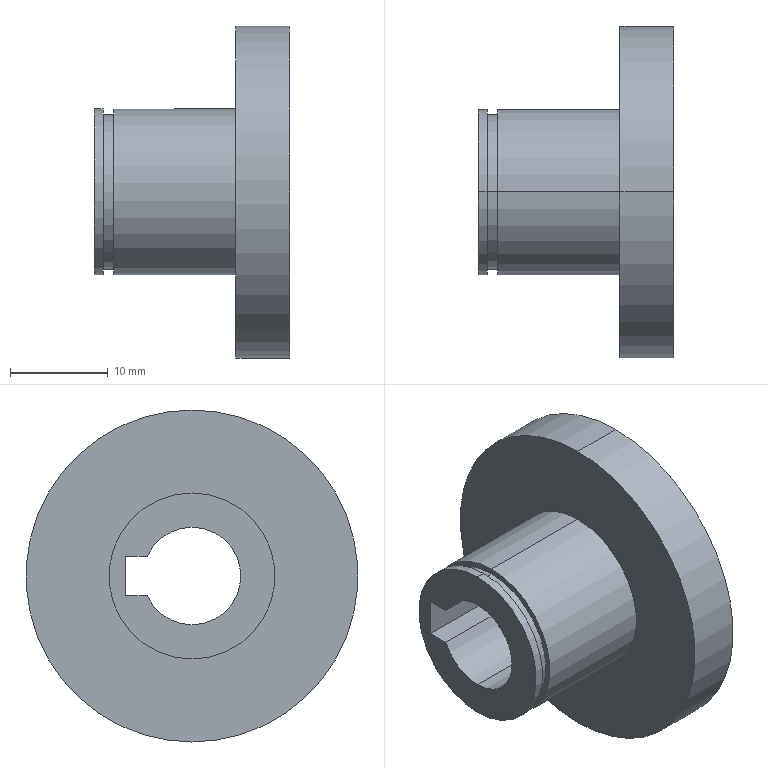Part | SolidWorks | features ICE 1, Revolution 1 | 1 solid | 25 faces | box 20 x 34 x 34 mm | volume 6019 mm3 | cylinder 15 | plane 10 | commonest cylinder face diameters 17 x4 10 x3 15.8 x2 16 x2 30 x2 34 x2
STEP:
#1=CARTESIAN_POINT('',(0.9,0.,8.5));
#2=VERTEX_POINT('',#1);
#3=CARTESIAN_POINT('',(0.9,0.,-8.5));
#4=VERTEX_POINT('',#3);
#5=CARTESIAN_POINT('',(0.9,0.,0.));
#6=DIRECTION('',(-1.,0.,0.));
#7=DIRECTION('',(0.,0.,1.));
#8=AXIS2_PLACEMENT_3D('',#5,#6,#7);
#9=CIRCLE('',#8,8.5);
#10=EDGE_CURVE('',#2,#4,#9,.T.);
#11=ORIENTED_EDGE('',*,*,#10,.T.);
#12=CARTESIAN_POINT('',(0.,0.,-8.5));
#13=VERTEX_POINT('',#12);
#14=CARTESIAN_POINT('',(0.,0.,-8.5));
#15=DIRECTION('',(-1.,0.,0.));
#16=VECTOR('',#15,1000.);
#17=LINE('',#14,#16);
#18=EDGE_CURVE('',#4,#13,#17,.T.);
#19=ORIENTED_EDGE('',*,*,#18,.T.);
#20=CARTESIAN_POINT('',(0.,0.,8.5));
#21=VERTEX_POINT('',#20);
#22=CARTESIAN_POINT('',(0.,0.,0.));
#23=DIRECTION('',(-1.,0.,0.));
#24=DIRECTION('',(0.,0.,1.));
#25=AXIS2_PLACEMENT_3D('',#22,#23,#24);
#26=CIRCLE('',#25,8.5);
#27=EDGE_CURVE('',#21,#13,#26,.T.);
#28=ORIENTED_EDGE('',*,*,#27,.F.);
#29=CARTESIAN_POINT('',(0.,0.,8.5));
#30=DIRECTION('',(-1.,0.,0.));
#31=VECTOR('',#30,1000.);
#32=LINE('',#29,#31);
#33=EDGE_CURVE('',#2,#21,#32,.T.);
#34=ORIENTED_EDGE('',*,*,#33,.F.);
#35=EDGE_LOOP('',(#11,#19,#28,#34));
#36=FACE_OUTER_BOUND('',#35,.T.);
#37=CARTESIAN_POINT('',(0.,0.,0.));
#38=DIRECTION('',(-1.,0.,0.));
#39=DIRECTION('',(0.,0.,1.));
#40=AXIS2_PLACEMENT_3D('',#37,#38,#39);
#41=CYLINDRICAL_SURFACE('',#40,8.5);
#42=ADVANCED_FACE('',(#36),#41,.T.);
#43=CARTESIAN_POINT('',(2.,0.,7.9));
#44=VERTEX_POINT('',#43);
#45=CARTESIAN_POINT('',(2.,0.,-7.9));
#46=VERTEX_POINT('',#45);
#47=CARTESIAN_POINT('',(2.,0.,0.));
#48=DIRECTION('',(-1.,0.,0.));
#49=DIRECTION('',(0.,0.,1.));
#50=AXIS2_PLACEMENT_3D('',#47,#48,#49);
#51=CIRCLE('',#50,7.9);
#52=EDGE_CURVE('',#44,#46,#51,.T.);
#53=ORIENTED_EDGE('',*,*,#52,.T.);
#54=CARTESIAN_POINT('',(0.9,0.,-7.9));
#55=VERTEX_POINT('',#54);
#56=CARTESIAN_POINT('',(0.,0.,-7.9));
#57=DIRECTION('',(-1.,0.,0.));
#58=VECTOR('',#57,1000.);
#59=LINE('',#56,#58);
#60=EDGE_CURVE('',#46,#55,#59,.T.);
#61=ORIENTED_EDGE('',*,*,#60,.T.);
#62=CARTESIAN_POINT('',(0.9,0.,7.9));
#63=VERTEX_POINT('',#62);
#64=CARTESIAN_POINT('',(0.9,0.,0.));
#65=DIRECTION('',(-1.,0.,0.));
#66=DIRECTION('',(0.,0.,1.));
#67=AXIS2_PLACEMENT_3D('',#64,#65,#66);
#68=CIRCLE('',#67,7.9);
#69=EDGE_CURVE('',#63,#55,#68,.T.);
#70=ORIENTED_EDGE('',*,*,#69,.F.);
#71=CARTESIAN_POINT('',(0.,0.,7.9));
#72=DIRECTION('',(-1.,0.,0.));
#73=VECTOR('',#72,1000.);
#74=LINE('',#71,#73);
#75=EDGE_CURVE('',#44,#63,#74,.T.);
#76=ORIENTED_EDGE('',*,*,#75,.F.);
#77=EDGE_LOOP('',(#53,#61,#70,#76));
#78=FACE_OUTER_BOUND('',#77,.T.);
#79=CARTESIAN_POINT('',(0.,0.,0.));
#80=DIRECTION('',(-1.,0.,0.));
#81=DIRECTION('',(0.,0.,1.));
#82=AXIS2_PLACEMENT_3D('',#79,#80,#81);
#83=CYLINDRICAL_SURFACE('',#82,7.9);
#84=ADVANCED_FACE('',(#78),#83,.T.);
#85=CARTESIAN_POINT('',(14.5,0.,8.5));
#86=VERTEX_POINT('',#85);
#87=CARTESIAN_POINT('',(14.5,0.,-8.5));
#88=VERTEX_POINT('',#87);
#89=CARTESIAN_POINT('',(14.5,0.,0.));
#90=DIRECTION('',(-1.,0.,0.));
#91=DIRECTION('',(0.,0.,1.));
#92=AXIS2_PLACEMENT_3D('',#89,#90,#91);
#93=CIRCLE('',#92,8.5);
#94=EDGE_CURVE('',#86,#88,#93,.T.);
#95=ORIENTED_EDGE('',*,*,#94,.T.);
#96=CARTESIAN_POINT('',(2.,0.,-8.5));
#97=VERTEX_POINT('',#96);
#98=CARTESIAN_POINT('',(0.,0.,-8.5));
#99=DIRECTION('',(-1.,0.,0.));
#100=VECTOR('',#99,1000.);
#101=LINE('',#98,#100);
#102=EDGE_CURVE('',#88,#97,#101,.T.);
#103=ORIENTED_EDGE('',*,*,#102,.T.);
#104=CARTESIAN_POINT('',(2.,0.,8.5));
#105=VERTEX_POINT('',#104);
#106=CARTESIAN_POINT('',(2.,0.,0.));
#107=DIRECTION('',(-1.,0.,0.));
#108=DIRECTION('',(0.,0.,1.));
#109=AXIS2_PLACEMENT_3D('',#106,#107,#108);
#110=CIRCLE('',#109,8.5);
#111=EDGE_CURVE('',#105,#97,#110,.T.);
#112=ORIENTED_EDGE('',*,*,#111,.F.);
#113=CARTESIAN_POINT('',(0.,0.,8.5));
#114=DIRECTION('',(-1.,0.,0.));
#115=VECTOR('',#114,1000.);
#116=LINE('',#113,#115);
#117=EDGE_CURVE('',#86,#105,#116,.T.);
#118=ORIENTED_EDGE('',*,*,#117,.F.);
#119=EDGE_LOOP('',(#95,#103,#112,#118));
#120=FACE_OUTER_BOUND('',#119,.T.);
#121=CARTESIAN_POINT('',(0.,0.,0.));
#122=DIRECTION('',(-1.,0.,0.));
#123=DIRECTION('',(0.,0.,1.));
#124=AXIS2_PLACEMENT_3D('',#121,#122,#123);
#125=CYLINDRICAL_SURFACE('',#124,8.5);
#126=ADVANCED_FACE('',(#120),#125,.T.);
#127=CARTESIAN_POINT('',(20.,0.,17.));
#128=VERTEX_POINT('',#127);
#129=CARTESIAN_POINT('',(20.,0.,-17.));
#130=VERTEX_POINT('',#129);
#131=CARTESIAN_POINT('',(20.,0.,0.));
#132=DIRECTION('',(-1.,0.,0.));
#133=DIRECTION('',(0.,0.,1.));
#134=AXIS2_PLACEMENT_3D('',#131,#132,#133);
#135=CIRCLE('',#134,17.);
#136=EDGE_CURVE('',#128,#130,#135,.T.);
#137=ORIENTED_EDGE('',*,*,#136,.T.);
#138=CARTESIAN_POINT('',(14.5,0.,-17.));
#139=VERTEX_POINT('',#138);
#140=CARTESIAN_POINT('',(0.,0.,-17.));
#141=DIRECTION('',(-1.,0.,0.));
#142=VECTOR('',#141,1000.);
#143=LINE('',#140,#142);
#144=EDGE_CURVE('',#130,#139,#143,.T.);
#145=ORIENTED_EDGE('',*,*,#144,.T.);
#146=CARTESIAN_POINT('',(14.5,0.,17.));
#147=VERTEX_POINT('',#146);
#148=CARTESIAN_POINT('',(14.5,0.,0.));
#149=DIRECTION('',(-1.,0.,0.));
#150=DIRECTION('',(0.,0.,1.));
#151=AXIS2_PLACEMENT_3D('',#148,#149,#150);
#152=CIRCLE('',#151,17.);
#153=EDGE_CURVE('',#147,#139,#152,.T.);
#154=ORIENTED_EDGE('',*,*,#153,.F.);
#155=CARTESIAN_POINT('',(0.,0.,17.));
#156=DIRECTION('',(-1.,0.,0.));
#157=VECTOR('',#156,1000.);
#158=LINE('',#155,#157);
#159=EDGE_CURVE('',#128,#147,#158,.T.);
#160=ORIENTED_EDGE('',*,*,#159,.F.);
#161=EDGE_LOOP('',(#137,#145,#154,#160));
#162=FACE_OUTER_BOUND('',#161,.T.);
#163=CARTESIAN_POINT('',(0.,0.,0.));
#164=DIRECTION('',(-1.,0.,0.));
#165=DIRECTION('',(0.,0.,1.));
#166=AXIS2_PLACEMENT_3D('',#163,#164,#165);
#167=CYLINDRICAL_SURFACE('',#166,17.);
#168=ADVANCED_FACE('',(#162),#167,.T.);
#169=CARTESIAN_POINT('',(20.,0.,-15.));
#170=VERTEX_POINT('',#169);
#171=CARTESIAN_POINT('',(20.,0.,15.));
#172=VERTEX_POINT('',#171);
#173=CARTESIAN_POINT('',(20.,0.,0.));
#174=DIRECTION('',(-1.,0.,0.));
#175=DIRECTION('',(0.,0.,1.));
#176=AXIS2_PLACEMENT_3D('',#173,#174,#175);
#177=CIRCLE('',#176,15.);
#178=EDGE_CURVE('',#170,#172,#177,.T.);
#179=ORIENTED_EDGE('',*,*,#178,.F.);
#180=CARTESIAN_POINT('',(19.,0.,-15.));
#181=VERTEX_POINT('',#180);
#182=CARTESIAN_POINT('',(0.,0.,-15.));
#183=DIRECTION('',(-1.,0.,0.));
#184=VECTOR('',#183,1000.);
#185=LINE('',#182,#184);
#186=EDGE_CURVE('',#170,#181,#185,.T.);
#187=ORIENTED_EDGE('',*,*,#186,.T.);
#188=CARTESIAN_POINT('',(19.,0.,15.));
#189=VERTEX_POINT('',#188);
#190=CARTESIAN_POINT('',(19.,0.,0.));
#191=DIRECTION('',(-1.,0.,0.));
#192=DIRECTION('',(0.,0.,1.));
#193=AXIS2_PLACEMENT_3D('',#190,#191,#192);
#194=CIRCLE('',#193,15.);
#195=EDGE_CURVE('',#181,#189,#194,.T.);
#196=ORIENTED_EDGE('',*,*,#195,.T.);
#197=CARTESIAN_POINT('',(0.,0.,15.));
#198=DIRECTION('',(-1.,0.,0.));
#199=VECTOR('',#198,1000.);
#200=LINE('',#197,#199);
#201=EDGE_CURVE('',#172,#189,#200,.T.);
#202=ORIENTED_EDGE('',*,*,#201,.F.);
#203=EDGE_LOOP('',(#179,#187,#196,#202));
#204=FACE_OUTER_BOUND('',#203,.T.);
#205=CARTESIAN_POINT('',(0.,0.,0.));
#206=DIRECTION('',(-1.,0.,0.));
#207=DIRECTION('',(0.,0.,1.));
#208=AXIS2_PLACEMENT_3D('',#205,#206,#207);
#209=CYLINDRICAL_SURFACE('',#208,15.);
#210=ADVANCED_FACE('',(#204),#209,.F.);
#211=CARTESIAN_POINT('',(20.,0.,8.));
#212=VERTEX_POINT('',#211);
#213=CARTESIAN_POINT('',(20.,0.,-8.));
#214=VERTEX_POINT('',#213);
#215=CARTESIAN_POINT('',(20.,0.,0.));
#216=DIRECTION('',(-1.,0.,0.));
#217=DIRECTION('',(0.,0.,1.));
#218=AXIS2_PLACEMENT_3D('',#215,#216,#217);
#219=CIRCLE('',#218,8.);
#220=EDGE_CURVE('',#212,#214,#219,.T.);
#221=ORIENTED_EDGE('',*,*,#220,.T.);
#222=CARTESIAN_POINT('',(19.,0.,-8.));
#223=VERTEX_POINT('',#222);
#224=CARTESIAN_POINT('',(0.,0.,-8.));
#225=DIRECTION('',(-1.,0.,0.));
#226=VECTOR('',#225,1000.);
#227=LINE('',#224,#226);
#228=EDGE_CURVE('',#214,#223,#227,.T.);
#229=ORIENTED_EDGE('',*,*,#228,.T.);
#230=CARTESIAN_POINT('',(19.,0.,8.));
#231=VERTEX_POINT('',#230);
#232=CARTESIAN_POINT('',(19.,0.,0.));
#233=DIRECTION('',(-1.,0.,0.));
#234=DIRECTION('',(0.,0.,1.));
#235=AXIS2_PLACEMENT_3D('',#232,#233,#234);
#236=CIRCLE('',#235,8.);
#237=EDGE_CURVE('',#231,#223,#236,.T.);
#238=ORIENTED_EDGE('',*,*,#237,.F.);
#239=CARTESIAN_POINT('',(0.,0.,8.));
#240=DIRECTION('',(-1.,0.,0.));
#241=VECTOR('',#240,1000.);
#242=LINE('',#239,#241);
#243=EDGE_CURVE('',#212,#231,#242,.T.);
#244=ORIENTED_EDGE('',*,*,#243,.F.);
#245=EDGE_LOOP('',(#221,#229,#238,#244));
#246=FACE_OUTER_BOUND('',#245,.T.);
#247=CARTESIAN_POINT('',(0.,0.,0.));
#248=DIRECTION('',(-1.,0.,0.));
#249=DIRECTION('',(0.,0.,1.));
#250=AXIS2_PLACEMENT_3D('',#247,#248,#249);
#251=CYLINDRICAL_SURFACE('',#250,8.);
#252=ADVANCED_FACE('',(#246),#251,.T.);
#253=CARTESIAN_POINT('',(20.,0.,-5.));
#254=VERTEX_POINT('',#253);
#255=CARTESIAN_POINT('',(20.,0.,5.));
#256=VERTEX_POINT('',#255);
#257=CARTESIAN_POINT('',(20.,0.,0.));
#258=DIRECTION('',(-1.,0.,0.));
#259=DIRECTION('',(0.,0.,1.));
#260=AXIS2_PLACEMENT_3D('',#257,#258,#259);
#261=CIRCLE('',#260,5.);
#262=EDGE_CURVE('',#254,#256,#261,.T.);
#263=ORIENTED_EDGE('',*,*,#262,.F.);
#264=CARTESIAN_POINT('',(0.,0.,-5.));
#265=VERTEX_POINT('',#264);
#266=CARTESIAN_POINT('',(0.,0.,-5.));
#267=DIRECTION('',(-1.,0.,0.));
#268=VECTOR('',#267,1000.);
#269=LINE('',#266,#268);
#270=EDGE_CURVE('',#254,#265,#269,.T.);
#271=ORIENTED_EDGE('',*,*,#270,.T.);
#272=CARTESIAN_POINT('',(0.,0.,5.));
#273=VERTEX_POINT('',#272);
#274=CARTESIAN_POINT('',(0.,0.,0.));
#275=DIRECTION('',(-1.,0.,0.));
#276=DIRECTION('',(0.,0.,1.));
#277=AXIS2_PLACEMENT_3D('',#274,#275,#276);
#278=CIRCLE('',#277,5.);
#279=EDGE_CURVE('',#265,#273,#278,.T.);
#280=ORIENTED_EDGE('',*,*,#279,.T.);
#281=CARTESIAN_POINT('',(0.,0.,5.));
#282=DIRECTION('',(-1.,0.,0.));
#283=VECTOR('',#282,1000.);
#284=LINE('',#281,#283);
#285=EDGE_CURVE('',#256,#273,#284,.T.);
#286=ORIENTED_EDGE('',*,*,#285,.F.);
#287=EDGE_LOOP('',(#263,#271,#280,#286));
#288=FACE_OUTER_BOUND('',#287,.T.);
#289=CARTESIAN_POINT('',(0.,0.,0.));
#290=DIRECTION('',(-1.,0.,0.));
#291=DIRECTION('',(0.,0.,1.));
#292=AXIS2_PLACEMENT_3D('',#289,#290,#291);
#293=CYLINDRICAL_SURFACE('',#292,5.);
#294=ADVANCED_FACE('',(#288),#293,.F.);
#295=CARTESIAN_POINT('',(20.,4.583,2.));
#296=VERTEX_POINT('',#295);
#297=CARTESIAN_POINT('',(20.,0.,0.));
#298=DIRECTION('',(-1.,0.,0.));
#299=DIRECTION('',(0.,0.,1.));
#300=AXIS2_PLACEMENT_3D('',#297,#298,#299);
#301=CIRCLE('',#300,5.);
#302=EDGE_CURVE('',#256,#296,#301,.T.);
#303=ORIENTED_EDGE('',*,*,#302,.F.);
#304=ORIENTED_EDGE('',*,*,#285,.T.);
#305=CARTESIAN_POINT('',(0.,4.583,2.));
#306=VERTEX_POINT('',#305);
#307=CARTESIAN_POINT('',(0.,0.,0.));
#308=DIRECTION('',(-1.,0.,0.));
#309=DIRECTION('',(0.,0.,1.));
#310=AXIS2_PLACEMENT_3D('',#307,#308,#309);
#311=CIRCLE('',#310,5.);
#312=EDGE_CURVE('',#273,#306,#311,.T.);
#313=ORIENTED_EDGE('',*,*,#312,.T.);
#314=CARTESIAN_POINT('',(0.,4.583,2.));
#315=DIRECTION('',(1.,0.,0.));
#316=VECTOR('',#315,1000.);
#317=LINE('',#314,#316);
#318=EDGE_CURVE('',#306,#296,#317,.T.);
#319=ORIENTED_EDGE('',*,*,#318,.T.);
#320=EDGE_LOOP('',(#303,#304,#313,#319));
#321=FACE_OUTER_BOUND('',#320,.T.);
#322=CARTESIAN_POINT('',(0.,0.,0.));
#323=DIRECTION('',(-1.,0.,0.));
#324=DIRECTION('',(0.,0.,1.));
#325=AXIS2_PLACEMENT_3D('',#322,#323,#324);
#326=CYLINDRICAL_SURFACE('',#325,5.);
#327=ADVANCED_FACE('',(#321),#326,.F.);
#328=CARTESIAN_POINT('',(0.,6.8,-2.));
#329=VERTEX_POINT('',#328);
#330=CARTESIAN_POINT('',(0.,6.8,2.));
#331=VERTEX_POINT('',#330);
#332=CARTESIAN_POINT('',(0.,6.8,2.));
#333=DIRECTION('',(0.,0.,1.));
#334=VECTOR('',#333,1000.);
#335=LINE('',#332,#334);
#336=EDGE_CURVE('',#329,#331,#335,.T.);
#337=ORIENTED_EDGE('',*,*,#336,.T.);
#338=CARTESIAN_POINT('',(0.,0.,2.));
#339=DIRECTION('',(0.,-1.,0.));
#340=VECTOR('',#339,1000.);
#341=LINE('',#338,#340);
#342=EDGE_CURVE('',#331,#306,#341,.T.);
#343=ORIENTED_EDGE('',*,*,#342,.T.);
#344=ORIENTED_EDGE('',*,*,#312,.F.);
#345=ORIENTED_EDGE('',*,*,#279,.F.);
#346=CARTESIAN_POINT('',(0.,4.583,-2.));
#347=VERTEX_POINT('',#346);
#348=CARTESIAN_POINT('',(0.,0.,0.));
#349=DIRECTION('',(-1.,0.,0.));
#350=DIRECTION('',(0.,0.,1.));
#351=AXIS2_PLACEMENT_3D('',#348,#349,#350);
#352=CIRCLE('',#351,5.);
#353=EDGE_CURVE('',#347,#265,#352,.T.);
#354=ORIENTED_EDGE('',*,*,#353,.F.);
#355=CARTESIAN_POINT('',(0.,0.,-2.));
#356=DIRECTION('',(0.,1.,0.));
#357=VECTOR('',#356,1000.);
#358=LINE('',#355,#357);
#359=EDGE_CURVE('',#347,#329,#358,.T.);
#360=ORIENTED_EDGE('',*,*,#359,.T.);
#361=EDGE_LOOP('',(#337,#343,#344,#345,#354,#360));
#362=FACE_BOUND('',#361,.T.);
#363=ORIENTED_EDGE('',*,*,#27,.T.);
#364=CARTESIAN_POINT('',(0.,0.,0.));
#365=DIRECTION('',(-1.,0.,0.));
#366=DIRECTION('',(0.,0.,1.));
#367=AXIS2_PLACEMENT_3D('',#364,#365,#366);
#368=CIRCLE('',#367,8.5);
#369=EDGE_CURVE('',#13,#21,#368,.T.);
#370=ORIENTED_EDGE('',*,*,#369,.T.);
#371=EDGE_LOOP('',(#363,#370));
#372=FACE_OUTER_BOUND('',#371,.T.);
#373=CARTESIAN_POINT('',(0.,8.5,0.));
#374=DIRECTION('',(1.,0.,0.));
#375=DIRECTION('',(0.,0.,-1.));
#376=AXIS2_PLACEMENT_3D('',#373,#374,#375);
#377=PLANE('',#376);
#378=ADVANCED_FACE('',(#362,#372),#377,.F.);
#379=ORIENTED_EDGE('',*,*,#270,.F.);
#380=CARTESIAN_POINT('',(20.,4.583,-2.));
#381=VERTEX_POINT('',#380);
#382=CARTESIAN_POINT('',(20.,0.,0.));
#383=DIRECTION('',(-1.,0.,0.));
#384=DIRECTION('',(0.,0.,1.));
#385=AXIS2_PLACEMENT_3D('',#382,#383,#384);
#386=CIRCLE('',#385,5.);
#387=EDGE_CURVE('',#381,#254,#386,.T.);
#388=ORIENTED_EDGE('',*,*,#387,.F.);
#389=CARTESIAN_POINT('',(0.,4.583,-2.));
#390=DIRECTION('',(-1.,0.,0.));
#391=VECTOR('',#390,1000.);
#392=LINE('',#389,#391);
#393=EDGE_CURVE('',#381,#347,#392,.T.);
#394=ORIENTED_EDGE('',*,*,#393,.T.);
#395=ORIENTED_EDGE('',*,*,#353,.T.);
#396=EDGE_LOOP('',(#379,#388,#394,#395));
#397=FACE_OUTER_BOUND('',#396,.T.);
#398=CARTESIAN_POINT('',(0.,0.,0.));
#399=DIRECTION('',(-1.,0.,0.));
#400=DIRECTION('',(0.,0.,1.));
#401=AXIS2_PLACEMENT_3D('',#398,#399,#400);
#402=CYLINDRICAL_SURFACE('',#401,5.);
#403=ADVANCED_FACE('',(#397),#402,.F.);
#404=ORIENTED_EDGE('',*,*,#220,.F.);
#405=CARTESIAN_POINT('',(20.,0.,0.));
#406=DIRECTION('',(-1.,0.,0.));
#407=DIRECTION('',(0.,0.,1.));
#408=AXIS2_PLACEMENT_3D('',#405,#406,#407);
#409=CIRCLE('',#408,8.);
#410=EDGE_CURVE('',#214,#212,#409,.T.);
#411=ORIENTED_EDGE('',*,*,#410,.F.);
#412=EDGE_LOOP('',(#404,#411));
#413=FACE_OUTER_BOUND('',#412,.T.);
#414=ORIENTED_EDGE('',*,*,#387,.T.);
#415=ORIENTED_EDGE('',*,*,#262,.T.);
#416=ORIENTED_EDGE('',*,*,#302,.T.);
#417=CARTESIAN_POINT('',(20.,6.8,2.));
#418=VERTEX_POINT('',#417);
#419=CARTESIAN_POINT('',(20.,0.,2.));
#420=DIRECTION('',(0.,-1.,0.));
#421=VECTOR('',#420,1000.);
#422=LINE('',#419,#421);
#423=EDGE_CURVE('',#418,#296,#422,.T.);
#424=ORIENTED_EDGE('',*,*,#423,.F.);
#425=CARTESIAN_POINT('',(20.,6.8,-2.));
#426=VERTEX_POINT('',#425);
#427=CARTESIAN_POINT('',(20.,6.8,2.));
#428=DIRECTION('',(0.,0.,1.));
#429=VECTOR('',#428,1000.);
#430=LINE('',#427,#429);
#431=EDGE_CURVE('',#426,#418,#430,.T.);
#432=ORIENTED_EDGE('',*,*,#431,.F.);
#433=CARTESIAN_POINT('',(20.,5.,-2.));
#434=DIRECTION('',(0.,-1.,0.));
#435=VECTOR('',#434,1000.);
#436=LINE('',#433,#435);
#437=EDGE_CURVE('',#426,#381,#436,.T.);
#438=ORIENTED_EDGE('',*,*,#437,.T.);
#439=EDGE_LOOP('',(#414,#415,#416,#424,#432,#438));
#440=FACE_BOUND('',#439,.T.);
#441=CARTESIAN_POINT('',(20.,5.,0.));
#442=DIRECTION('',(-1.,0.,0.));
#443=DIRECTION('',(0.,0.,1.));
#444=AXIS2_PLACEMENT_3D('',#441,#442,#443);
#445=PLANE('',#444);
#446=ADVANCED_FACE('',(#413,#440),#445,.F.);
#447=ORIENTED_EDGE('',*,*,#228,.F.);
#448=ORIENTED_EDGE('',*,*,#410,.T.);
#449=ORIENTED_EDGE('',*,*,#243,.T.);
#450=CARTESIAN_POINT('',(19.,0.,0.));
#451=DIRECTION('',(-1.,0.,0.));
#452=DIRECTION('',(0.,0.,1.));
#453=AXIS2_PLACEMENT_3D('',#450,#451,#452);
#454=CIRCLE('',#453,8.);
#455=EDGE_CURVE('',#223,#231,#454,.T.);
#456=ORIENTED_EDGE('',*,*,#455,.F.);
#457=EDGE_LOOP('',(#447,#448,#449,#456));
#458=FACE_OUTER_BOUND('',#457,.T.);
#459=CARTESIAN_POINT('',(0.,0.,0.));
#460=DIRECTION('',(-1.,0.,0.));
#461=DIRECTION('',(0.,0.,1.));
#462=AXIS2_PLACEMENT_3D('',#459,#460,#461);
#463=CYLINDRICAL_SURFACE('',#462,8.);
#464=ADVANCED_FACE('',(#458),#463,.T.);
#465=CARTESIAN_POINT('',(19.,0.,0.));
#466=DIRECTION('',(-1.,0.,0.));
#467=DIRECTION('',(0.,0.,1.));
#468=AXIS2_PLACEMENT_3D('',#465,#466,#467);
#469=CIRCLE('',#468,15.);
#470=EDGE_CURVE('',#189,#181,#469,.T.);
#471=ORIENTED_EDGE('',*,*,#470,.F.);
#472=ORIENTED_EDGE('',*,*,#195,.F.);
#473=EDGE_LOOP('',(#471,#472));
#474=FACE_OUTER_BOUND('',#473,.T.);
#475=ORIENTED_EDGE('',*,*,#237,.T.);
#476=ORIENTED_EDGE('',*,*,#455,.T.);
#477=EDGE_LOOP('',(#475,#476));
#478=FACE_BOUND('',#477,.T.);
#479=CARTESIAN_POINT('',(19.,8.,0.));
#480=DIRECTION('',(-1.,0.,0.));
#481=DIRECTION('',(0.,0.,1.));
#482=AXIS2_PLACEMENT_3D('',#479,#480,#481);
#483=PLANE('',#482);
#484=ADVANCED_FACE('',(#474,#478),#483,.F.);
#485=ORIENTED_EDGE('',*,*,#186,.F.);
#486=CARTESIAN_POINT('',(20.,0.,0.));
#487=DIRECTION('',(-1.,0.,0.));
#488=DIRECTION('',(0.,0.,1.));
#489=AXIS2_PLACEMENT_3D('',#486,#487,#488);
#490=CIRCLE('',#489,15.);
#491=EDGE_CURVE('',#172,#170,#490,.T.);
#492=ORIENTED_EDGE('',*,*,#491,.F.);
#493=ORIENTED_EDGE('',*,*,#201,.T.);
#494=ORIENTED_EDGE('',*,*,#470,.T.);
#495=EDGE_LOOP('',(#485,#492,#493,#494));
#496=FACE_OUTER_BOUND('',#495,.T.);
#497=CARTESIAN_POINT('',(0.,0.,0.));
#498=DIRECTION('',(-1.,0.,0.));
#499=DIRECTION('',(0.,0.,1.));
#500=AXIS2_PLACEMENT_3D('',#497,#498,#499);
#501=CYLINDRICAL_SURFACE('',#500,15.);
#502=ADVANCED_FACE('',(#496),#501,.F.);
#503=ORIENTED_EDGE('',*,*,#136,.F.);
#504=CARTESIAN_POINT('',(20.,0.,0.));
#505=DIRECTION('',(-1.,0.,0.));
#506=DIRECTION('',(0.,0.,1.));
#507=AXIS2_PLACEMENT_3D('',#504,#505,#506);
#508=CIRCLE('',#507,17.);
#509=EDGE_CURVE('',#130,#128,#508,.T.);
#510=ORIENTED_EDGE('',*,*,#509,.F.);
#511=EDGE_LOOP('',(#503,#510));
#512=FACE_OUTER_BOUND('',#511,.T.);
#513=ORIENTED_EDGE('',*,*,#491,.T.);
#514=ORIENTED_EDGE('',*,*,#178,.T.);
#515=EDGE_LOOP('',(#513,#514));
#516=FACE_BOUND('',#515,.T.);
#517=CARTESIAN_POINT('',(20.,15.,0.));
#518=DIRECTION('',(-1.,0.,0.));
#519=DIRECTION('',(0.,0.,1.));
#520=AXIS2_PLACEMENT_3D('',#517,#518,#519);
#521=PLANE('',#520);
#522=ADVANCED_FACE('',(#512,#516),#521,.F.);
#523=ORIENTED_EDGE('',*,*,#144,.F.);
#524=ORIENTED_EDGE('',*,*,#509,.T.);
#525=ORIENTED_EDGE('',*,*,#159,.T.);
#526=CARTESIAN_POINT('',(14.5,0.,0.));
#527=DIRECTION('',(-1.,0.,0.));
#528=DIRECTION('',(0.,0.,1.));
#529=AXIS2_PLACEMENT_3D('',#526,#527,#528);
#530=CIRCLE('',#529,17.);
#531=EDGE_CURVE('',#139,#147,#530,.T.);
#532=ORIENTED_EDGE('',*,*,#531,.F.);
#533=EDGE_LOOP('',(#523,#524,#525,#532));
#534=FACE_OUTER_BOUND('',#533,.T.);
#535=CARTESIAN_POINT('',(0.,0.,0.));
#536=DIRECTION('',(-1.,0.,0.));
#537=DIRECTION('',(0.,0.,1.));
#538=AXIS2_PLACEMENT_3D('',#535,#536,#537);
#539=CYLINDRICAL_SURFACE('',#538,17.);
#540=ADVANCED_FACE('',(#534),#539,.T.);
#541=ORIENTED_EDGE('',*,*,#94,.F.);
#542=CARTESIAN_POINT('',(14.5,0.,0.));
#543=DIRECTION('',(-1.,0.,0.));
#544=DIRECTION('',(0.,0.,1.));
#545=AXIS2_PLACEMENT_3D('',#542,#543,#544);
#546=CIRCLE('',#545,8.5);
#547=EDGE_CURVE('',#88,#86,#546,.T.);
#548=ORIENTED_EDGE('',*,*,#547,.F.);
#549=EDGE_LOOP('',(#541,#548));
#550=FACE_BOUND('',#549,.T.);
#551=ORIENTED_EDGE('',*,*,#153,.T.);
#552=ORIENTED_EDGE('',*,*,#531,.T.);
#553=EDGE_LOOP('',(#551,#552));
#554=FACE_OUTER_BOUND('',#553,.T.);
#555=CARTESIAN_POINT('',(14.5,17.,0.));
#556=DIRECTION('',(1.,0.,0.));
#557=DIRECTION('',(0.,0.,-1.));
#558=AXIS2_PLACEMENT_3D('',#555,#556,#557);
#559=PLANE('',#558);
#560=ADVANCED_FACE('',(#550,#554),#559,.F.);
#561=ORIENTED_EDGE('',*,*,#102,.F.);
#562=ORIENTED_EDGE('',*,*,#547,.T.);
#563=ORIENTED_EDGE('',*,*,#117,.T.);
#564=CARTESIAN_POINT('',(2.,0.,0.));
#565=DIRECTION('',(-1.,0.,0.));
#566=DIRECTION('',(0.,0.,1.));
#567=AXIS2_PLACEMENT_3D('',#564,#565,#566);
#568=CIRCLE('',#567,8.5);
#569=EDGE_CURVE('',#97,#105,#568,.T.);
#570=ORIENTED_EDGE('',*,*,#569,.F.);
#571=EDGE_LOOP('',(#561,#562,#563,#570));
#572=FACE_OUTER_BOUND('',#571,.T.);
#573=CARTESIAN_POINT('',(0.,0.,0.));
#574=DIRECTION('',(-1.,0.,0.));
#575=DIRECTION('',(0.,0.,1.));
#576=AXIS2_PLACEMENT_3D('',#573,#574,#575);
#577=CYLINDRICAL_SURFACE('',#576,8.5);
#578=ADVANCED_FACE('',(#572),#577,.T.);
#579=ORIENTED_EDGE('',*,*,#52,.F.);
#580=CARTESIAN_POINT('',(2.,0.,0.));
#581=DIRECTION('',(-1.,0.,0.));
#582=DIRECTION('',(0.,0.,1.));
#583=AXIS2_PLACEMENT_3D('',#580,#581,#582);
#584=CIRCLE('',#583,7.9);
#585=EDGE_CURVE('',#46,#44,#584,.T.);
#586=ORIENTED_EDGE('',*,*,#585,.F.);
#587=EDGE_LOOP('',(#579,#586));
#588=FACE_BOUND('',#587,.T.);
#589=ORIENTED_EDGE('',*,*,#111,.T.);
#590=ORIENTED_EDGE('',*,*,#569,.T.);
#591=EDGE_LOOP('',(#589,#590));
#592=FACE_OUTER_BOUND('',#591,.T.);
#593=CARTESIAN_POINT('',(2.,8.5,0.));
#594=DIRECTION('',(1.,0.,0.));
#595=DIRECTION('',(0.,0.,-1.));
#596=AXIS2_PLACEMENT_3D('',#593,#594,#595);
#597=PLANE('',#596);
#598=ADVANCED_FACE('',(#588,#592),#597,.F.);
#599=ORIENTED_EDGE('',*,*,#60,.F.);
#600=ORIENTED_EDGE('',*,*,#585,.T.);
#601=ORIENTED_EDGE('',*,*,#75,.T.);
#602=CARTESIAN_POINT('',(0.9,0.,0.));
#603=DIRECTION('',(-1.,0.,0.));
#604=DIRECTION('',(0.,0.,1.));
#605=AXIS2_PLACEMENT_3D('',#602,#603,#604);
#606=CIRCLE('',#605,7.9);
#607=EDGE_CURVE('',#55,#63,#606,.T.);
#608=ORIENTED_EDGE('',*,*,#607,.F.);
#609=EDGE_LOOP('',(#599,#600,#601,#608));
#610=FACE_OUTER_BOUND('',#609,.T.);
#611=CARTESIAN_POINT('',(0.,0.,0.));
#612=DIRECTION('',(-1.,0.,0.));
#613=DIRECTION('',(0.,0.,1.));
#614=AXIS2_PLACEMENT_3D('',#611,#612,#613);
#615=CYLINDRICAL_SURFACE('',#614,7.9);
#616=ADVANCED_FACE('',(#610),#615,.T.);
#617=ORIENTED_EDGE('',*,*,#10,.F.);
#618=CARTESIAN_POINT('',(0.9,0.,0.));
#619=DIRECTION('',(-1.,0.,0.));
#620=DIRECTION('',(0.,0.,1.));
#621=AXIS2_PLACEMENT_3D('',#618,#619,#620);
#622=CIRCLE('',#621,8.5);
#623=EDGE_CURVE('',#4,#2,#622,.T.);
#624=ORIENTED_EDGE('',*,*,#623,.F.);
#625=EDGE_LOOP('',(#617,#624));
#626=FACE_OUTER_BOUND('',#625,.T.);
#627=ORIENTED_EDGE('',*,*,#69,.T.);
#628=ORIENTED_EDGE('',*,*,#607,.T.);
#629=EDGE_LOOP('',(#627,#628));
#630=FACE_BOUND('',#629,.T.);
#631=CARTESIAN_POINT('',(0.9,7.9,0.));
#632=DIRECTION('',(-1.,0.,0.));
#633=DIRECTION('',(0.,0.,1.));
#634=AXIS2_PLACEMENT_3D('',#631,#632,#633);
#635=PLANE('',#634);
#636=ADVANCED_FACE('',(#626,#630),#635,.F.);
#637=ORIENTED_EDGE('',*,*,#18,.F.);
#638=ORIENTED_EDGE('',*,*,#623,.T.);
#639=ORIENTED_EDGE('',*,*,#33,.T.);
#640=ORIENTED_EDGE('',*,*,#369,.F.);
#641=EDGE_LOOP('',(#637,#638,#639,#640));
#642=FACE_OUTER_BOUND('',#641,.T.);
#643=CARTESIAN_POINT('',(0.,0.,0.));
#644=DIRECTION('',(-1.,0.,0.));
#645=DIRECTION('',(0.,0.,1.));
#646=AXIS2_PLACEMENT_3D('',#643,#644,#645);
#647=CYLINDRICAL_SURFACE('',#646,8.5);
#648=ADVANCED_FACE('',(#642),#647,.T.);
#649=ORIENTED_EDGE('',*,*,#342,.F.);
#650=CARTESIAN_POINT('',(0.,6.8,2.));
#651=DIRECTION('',(1.,0.,0.));
#652=VECTOR('',#651,1000.);
#653=LINE('',#650,#652);
#654=EDGE_CURVE('',#331,#418,#653,.T.);
#655=ORIENTED_EDGE('',*,*,#654,.T.);
#656=ORIENTED_EDGE('',*,*,#423,.T.);
#657=ORIENTED_EDGE('',*,*,#318,.F.);
#658=EDGE_LOOP('',(#649,#655,#656,#657));
#659=FACE_OUTER_BOUND('',#658,.T.);
#660=CARTESIAN_POINT('',(0.,0.,2.));
#661=DIRECTION('',(0.,0.,1.));
#662=DIRECTION('',(1.,0.,0.));
#663=AXIS2_PLACEMENT_3D('',#660,#661,#662);
#664=PLANE('',#663);
#665=ADVANCED_FACE('',(#659),#664,.F.);
#666=ORIENTED_EDGE('',*,*,#437,.F.);
#667=CARTESIAN_POINT('',(0.,6.8,-2.));
#668=DIRECTION('',(1.,0.,0.));
#669=VECTOR('',#668,1000.);
#670=LINE('',#667,#669);
#671=EDGE_CURVE('',#329,#426,#670,.T.);
#672=ORIENTED_EDGE('',*,*,#671,.F.);
#673=ORIENTED_EDGE('',*,*,#359,.F.);
#674=ORIENTED_EDGE('',*,*,#393,.F.);
#675=EDGE_LOOP('',(#666,#672,#673,#674));
#676=FACE_OUTER_BOUND('',#675,.T.);
#677=CARTESIAN_POINT('',(0.,0.,-2.));
#678=DIRECTION('',(0.,0.,-1.));
#679=DIRECTION('',(-1.,0.,0.));
#680=AXIS2_PLACEMENT_3D('',#677,#678,#679);
#681=PLANE('',#680);
#682=ADVANCED_FACE('',(#676),#681,.F.);
#683=ORIENTED_EDGE('',*,*,#431,.T.);
#684=ORIENTED_EDGE('',*,*,#654,.F.);
#685=ORIENTED_EDGE('',*,*,#336,.F.);
#686=ORIENTED_EDGE('',*,*,#671,.T.);
#687=EDGE_LOOP('',(#683,#684,#685,#686));
#688=FACE_OUTER_BOUND('',#687,.T.);
#689=CARTESIAN_POINT('',(0.,6.8,2.));
#690=DIRECTION('',(0.,1.,0.));
#691=DIRECTION('',(0.,0.,1.));
#692=AXIS2_PLACEMENT_3D('',#689,#690,#691);
#693=PLANE('',#692);
#694=ADVANCED_FACE('',(#688),#693,.F.);
#695=CLOSED_SHELL('',(#42,#84,#126,#168,#210,#252,#294,#327,#378,#403,#446,#464,#484,#502,#522,#540,#560,#578,#598,#616,#636,#648,#665,#682,#694));
#696=MANIFOLD_SOLID_BREP('',#695);
#697=CARTESIAN_POINT('',(0.,0.,0.));
#698=DIRECTION('',(0.,0.,1.));
#699=DIRECTION('',(1.,0.,0.));
#700=AXIS2_PLACEMENT_3D('',#697,#698,#699);
#701=(LENGTH_UNIT()NAMED_UNIT(*)SI_UNIT(.MILLI.,.METRE.));
#702=UNCERTAINTY_MEASURE_WITH_UNIT(LENGTH_MEASURE(0.00001),#701,'','');
#703=(NAMED_UNIT(*)PLANE_ANGLE_UNIT()SI_UNIT($,.RADIAN.));
#704=(NAMED_UNIT(*)SI_UNIT($,.STERADIAN.)SOLID_ANGLE_UNIT());
#705=(GEOMETRIC_REPRESENTATION_CONTEXT(3)GLOBAL_UNCERTAINTY_ASSIGNED_CONTEXT((#702))GLOBAL_UNIT_ASSIGNED_CONTEXT((#701,#703,#704))REPRESENTATION_CONTEXT('',''));
#706=ADVANCED_BREP_SHAPE_REPRESENTATION('',(#696,#700),#705);